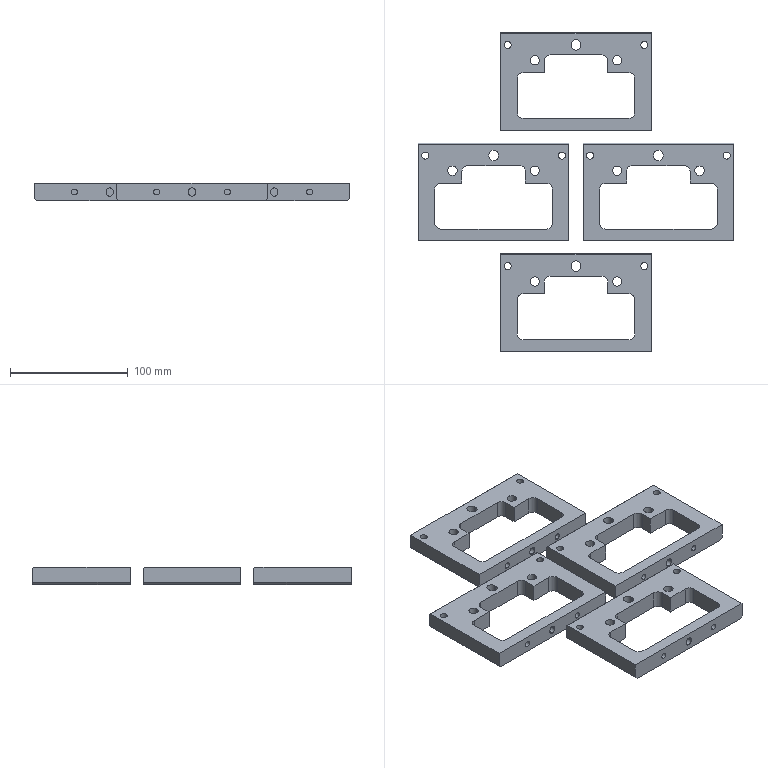NC program | NX | posted with a generic post | part box 268 x 271 x 15 mm
Lines 1946 to 2286 of 2286:
(PLANAR_MILL_1_COPY , TOOL : D6A45)
N3878 T07 M6
N3880 G54
N3882 G17 G0 G90 X31.063 Y-0.325 B0. C0. S9500 M3
N3884 G43 Z30. H7
N3886 Z0.
N3888 G94 G1 X31.1 Y-0.259 Z-0.02 F1250.
N3890 Y0. Z-0.09
N3892 Y0.259 Z-0.159
N3894 X30.799 Y0.799 Z-0.325
N3896 X30.259 Y1.1 Z-0.491
N3898 X29.741 Z-0.629
N3900 X29.201 Y0.799 Z-0.795
N3902 X28.9 Y0.259 Z-0.961
N3904 Y-0.259 Z-1.099
N3906 X29.201 Y-0.799 Z-1.265
N3908 X29.741 Y-1.1 Z-1.431
N3910 X30. Z-1.5
N3912 G3 X31.1 Y0. R1.1
N3914 X30. Y-1.1 R-1.1
N3916 X30.866 Y-0.6 R1.
N3918 G1 Z0.
N3920 G0 Z30.
N3922 X0.38 Y-0.626
N3924 Z0.
N3926 G1 Z-1.5
N3928 X1.1 Y-0.866
N3930 G3 X1.6 Y0. R1.
N3932 G1 Y0.5
N3934 G3 X0. Y2.1 R1.6
N3936 X-1.6 Y0.5 R1.6
N3938 G1 Y-0.5
N3940 G3 X0. Y-2.1 R1.6
N3942 X1.6 Y-0.5 R1.6
N3944 G1 Y0.
N3946 G3 X1.1 Y0.866 R1.
N3948 G1 X0.38 Y0.626
N3950 Z0.
N3952 G0 Z30.
N3954 X-28.937 Y-0.325
N3956 Z0.
N3958 G1 X-28.9 Y-0.259 Z-0.02
N3960 Y0. Z-0.09
N3962 Y0.259 Z-0.159
N3964 X-29.201 Y0.799 Z-0.325
N3966 X-29.741 Y1.1 Z-0.491
N3968 X-30.259 Z-0.629
N3970 X-30.799 Y0.799 Z-0.795
N3972 X-31.1 Y0.259 Z-0.961
N3974 Y-0.259 Z-1.099
N3976 X-30.799 Y-0.799 Z-1.265
N3978 X-30.259 Y-1.1 Z-1.431
N3980 X-30. Z-1.5
N3982 G3 X-28.9 Y0. R1.1
N3984 X-30. Y-1.1 R-1.1
N3986 X-29.134 Y-0.6 R1.
N3988 G1 Z0.
N3990 G0 Z30.
N3992 M5
(TOOLCOMP4_COPY , TOOL : D4)
N3994 T04 M6
N3996 G54
N3998 G17 G0 G90 X-0.499 Y0.731 B0. C0. S9500 M3
N4000 G43 Z30. H4
N4002 Z-0.333
N4004 G94 G1 Z-1.333 F1000.
N4006 G41 X-0.75 Y0.846 D4
N4008 G3 X-0.95 Y0.5 R0.4
N4010 G1 Y-0.5 F1200.
N4012 G3 X0. Y-1.45 R0.95
N4014 X0.95 Y-0.5 R0.95
N4016 G1 Y0.5
N4018 G3 X0. Y1.45 R0.95
N4020 X-0.95 Y0.5 R0.95
N4022 G1 Y-0.354 Z-1.524
N4024 X-0.944 Y-0.496 Z-1.556
N4026 X-0.933 Y-0.637 Z-1.587
N4028 X-0.91 Y-0.741 Z-1.611
N4030 X-0.897 Y-0.793 Z-1.623
N4032 X-0.882 Y-0.831 Z-1.632
N4034 X-0.85 Y-0.906 Z-1.651
N4036 X-0.795 Y-1.004 Z-1.676
N4038 X-0.765 Y-1.052 Z-1.689
N4040 X-0.741 Y-1.081 Z-1.697
N4042 X-0.692 Y-1.138 Z-1.714
N4044 X-0.609 Y-1.217 Z-1.74
N4046 X-0.566 Y-1.254 Z-1.753
N4048 X-0.536 Y-1.276 Z-1.761
N4050 X-0.473 Y-1.314 Z-1.778
N4052 X-0.365 Y-1.367 Z-1.805
N4054 X-0.31 Y-1.39 Z-1.818
N4056 X-0.278 Y-1.401 Z-1.826
N4058 X-0.212 Y-1.417 Z-1.841
N4060 X-0.09 Y-1.436 Z-1.869
N4062 X0.003 Y-1.443 Z-1.89
N4064 X0.069 Y-1.439 Z-1.905
N4066 X0.193 Y-1.421 Z-1.933
N4068 X0.284 Y-1.399 Z-1.954
N4070 X0.342 Y-1.377 Z-1.968
N4072 X0.457 Y-1.323 Z-1.997
N4074 X0.537 Y-1.274 Z-2.018
N4076 X0.586 Y-1.237 Z-2.032
N4078 X0.677 Y-1.157 Z-2.059
N4080 X0.738 Y-1.086 Z-2.08
N4082 X0.778 Y-1.031 Z-2.095
N4084 X0.838 Y-0.933 Z-2.121
N4086 X0.875 Y-0.847 Z-2.142
N4088 X0.901 Y-0.778 Z-2.159
N4090 X0.926 Y-0.672 Z-2.183
N4092 X0.935 Y-0.615 Z-2.196
N4094 X0.944 Y-0.5 Z-2.222
N4096 X0.95 Y-0.358 Z-2.254
N4098 Y0.354 Z-2.413
N4100 X0.944 Y0.496 Z-2.444
N4102 X0.933 Y0.637 Z-2.476
N4104 X0.91 Y0.741 Z-2.5
N4106 X0.897 Y0.793 Z-2.512
N4108 X0.85 Y0.906 Z-2.54
N4110 X0.798 Y1. Z-2.564
N4112 X0.77 Y1.045 Z-2.576
N4114 X0.744 Y1.077 Z-2.585
N4116 X0.692 Y1.138 Z-2.603
N4118 X0.588 Y1.235 Z-2.635
N4120 X0.477 Y1.321 Z-2.667
N4122 G3 X-0.95 Y0.5 R0.95
N4124 G1 Y-0.354 Z-2.857
N4126 X-0.944 Y-0.496 Z-2.889
N4128 X-0.933 Y-0.637 Z-2.921
N4130 X-0.909 Y-0.742 Z-2.945
N4132 X-0.897 Y-0.795 Z-2.957
N4134 X-0.85 Y-0.906 Z-2.984
N4136 X-0.795 Y-1.004 Z-3.009
N4138 X-0.766 Y-1.052 Z-3.022
N4140 X-0.692 Y-1.138 Z-3.048
N4142 X-0.609 Y-1.217 Z-3.073
N4144 X-0.566 Y-1.254 Z-3.086
N4146 X-0.536 Y-1.275 Z-3.094
N4148 X-0.473 Y-1.314 Z-3.111
N4150 X-0.365 Y-1.367 Z-3.138
N4152 X-0.31 Y-1.39 Z-3.151
N4154 X-0.278 Y-1.401 Z-3.159
N4156 X-0.212 Y-1.417 Z-3.175
N4158 X-0.091 Y-1.436 Z-3.202
N4160 X0.003 Y-1.443 Z-3.223
N4162 X0.068 Y-1.438 Z-3.238
N4164 X0.192 Y-1.421 Z-3.266
N4166 X0.284 Y-1.399 Z-3.287
N4168 X0.342 Y-1.376 Z-3.302
N4170 X0.457 Y-1.323 Z-3.33
N4172 X0.537 Y-1.275 Z-3.351
N4174 X0.586 Y-1.237 Z-3.365
N4176 X0.676 Y-1.157 Z-3.392
N4178 X0.737 Y-1.086 Z-3.413
N4180 X0.778 Y-1.031 Z-3.429
N4182 X0.838 Y-0.933 Z-3.454
N4184 X0.874 Y-0.847 Z-3.475
N4186 X0.901 Y-0.778 Z-3.492
N4188 X0.926 Y-0.673 Z-3.517
N4190 X0.935 Y-0.616 Z-3.53
N4192 X0.944 Y-0.5 Z-3.556
N4194 X0.95 Y-0.358 Z-3.587
N4196 Y0.354 Z-3.746
N4198 X0.944 Y0.496 Z-3.778
N4200 X0.933 Y0.637 Z-3.81
N4202 X0.909 Y0.742 Z-3.834
N4204 X0.897 Y0.795 Z-3.846
N4206 X0.85 Y0.906 Z-3.873
N4208 X0.798 Y0.999 Z-3.897
N4210 X0.77 Y1.045 Z-3.909
N4212 X0.745 Y1.077 Z-3.918
N4214 X0.692 Y1.138 Z-3.937
N4216 X0.588 Y1.234 Z-3.968
N4218 X0.477 Y1.321 Z-4.
N4220 G3 X-0.95 Y0.5 R0.95
N4222 G1 Y-0.354 Z-4.19
N4224 X-0.944 Y-0.496 Z-4.222
N4226 X-0.933 Y-0.637 Z-4.254
N4228 X-0.909 Y-0.742 Z-4.278
N4230 X-0.897 Y-0.794 Z-4.29
N4232 X-0.85 Y-0.906 Z-4.317
N4234 X-0.795 Y-1.004 Z-4.343
N4236 X-0.766 Y-1.051 Z-4.355
N4238 X-0.692 Y-1.138 Z-4.381
N4240 X-0.609 Y-1.217 Z-4.407
N4242 X-0.566 Y-1.254 Z-4.419
N4244 X-0.536 Y-1.275 Z-4.428
N4246 X-0.473 Y-1.314 Z-4.444
N4248 X-0.366 Y-1.367 Z-4.471
N4250 X-0.311 Y-1.389 Z-4.485
N4252 X-0.278 Y-1.4 Z-4.492
N4254 X-0.211 Y-1.417 Z-4.508
N4256 X-0.091 Y-1.436 Z-4.535
N4258 X0.002 Y-1.444 Z-4.556
N4260 X0.068 Y-1.438 Z-4.571
N4262 X0.195 Y-1.421 Z-4.6
N4264 X0.286 Y-1.399 Z-4.621
N4266 X0.342 Y-1.376 Z-4.635
N4268 X0.459 Y-1.322 Z-4.664
N4270 X0.539 Y-1.273 Z-4.685
N4272 X0.586 Y-1.237 Z-4.698
N4274 X0.677 Y-1.155 Z-4.726
N4276 X0.738 Y-1.084 Z-4.747
N4278 X0.778 Y-1.031 Z-4.762
N4280 X0.838 Y-0.934 Z-4.787
N4282 X0.874 Y-0.847 Z-4.809
N4284 X0.901 Y-0.778 Z-4.825
N4286 X0.926 Y-0.674 Z-4.85
N4288 X0.934 Y-0.616 Z-4.863
N4290 X0.944 Y-0.5 Z-4.889
N4292 X0.95 Y-0.358 Z-4.921
N4294 Y0.354 Z-5.079
N4296 X0.944 Y0.496 Z-5.111
N4298 X0.933 Y0.637 Z-5.143
N4300 X0.91 Y0.742 Z-5.167
N4302 X0.896 Y0.794 Z-5.179
N4304 X0.85 Y0.906 Z-5.206
N4306 X0.798 Y0.999 Z-5.23
N4308 X0.77 Y1.044 Z-5.242
N4310 X0.745 Y1.076 Z-5.252
N4312 X0.692 Y1.138 Z-5.27
N4314 X0.589 Y1.235 Z-5.302
N4316 X0.477 Y1.321 Z-5.333
N4318 G3 X-0.95 Y0.5 R0.95
N4320 G1 Y-0.354 Z-5.524
N4322 X-0.944 Y-0.496 Z-5.556
N4324 X-0.933 Y-0.637 Z-5.587
N4326 X-0.909 Y-0.742 Z-5.611
N4328 X-0.896 Y-0.794 Z-5.624
N4330 X-0.85 Y-0.906 Z-5.651
N4332 X-0.795 Y-1.003 Z-5.676
N4334 X-0.766 Y-1.051 Z-5.689
N4336 X-0.742 Y-1.08 Z-5.697
N4338 X-0.692 Y-1.138 Z-5.714
N4340 X-0.608 Y-1.218 Z-5.74
N4342 X-0.564 Y-1.255 Z-5.753
N4344 X-0.534 Y-1.276 Z-5.761
N4346 X-0.473 Y-1.313 Z-5.778
N4348 X-0.366 Y-1.366 Z-5.804
N4350 X-0.311 Y-1.389 Z-5.818
N4352 X-0.279 Y-1.4 Z-5.826
N4354 X-0.211 Y-1.417 Z-5.841
N4356 X-0.092 Y-1.436 Z-5.868
N4358 X0.002 Y-1.443 Z-5.89
N4360 X0.068 Y-1.438 Z-5.905
N4362 X0.194 Y-1.421 Z-5.933
N4364 X0.285 Y-1.399 Z-5.954
N4366 X0.342 Y-1.376 Z-5.968
N4368 X0.458 Y-1.322 Z-5.997
N4370 X0.538 Y-1.274 Z-6.018
N4372 X0.586 Y-1.237 Z-6.032
N4374 X0.677 Y-1.155 Z-6.059
N4376 X0.738 Y-1.084 Z-6.08
N4378 X0.778 Y-1.031 Z-6.095
N4380 X0.837 Y-0.934 Z-6.121
N4382 X0.874 Y-0.848 Z-6.142
N4384 X0.9 Y-0.778 Z-6.159
N4386 X0.918 Y-0.707 Z-6.175
N4388 X0.926 Y-0.671 Z-6.184
N4390 X0.935 Y-0.615 Z-6.196
N4392 X0.943 Y-0.5 Z-6.222
N4394 X0.95 Y-0.358 Z-6.254
N4396 Y0.354 Z-6.413
N4398 X0.944 Y0.496 Z-6.444
N4400 X0.933 Y0.637 Z-6.476
N4402 X0.909 Y0.742 Z-6.5
N4404 X0.896 Y0.794 Z-6.512
N4406 X0.85 Y0.906 Z-6.54
N4408 X0.798 Y0.998 Z-6.564
N4410 X0.77 Y1.044 Z-6.576
N4412 X0.745 Y1.076 Z-6.585
N4414 X0.692 Y1.138 Z-6.603
N4416 X0.588 Y1.235 Z-6.635
N4418 X0.477 Y1.321 Z-6.667
N4420 G3 X-0.95 Y0.5 R0.95
N4422 G1 Y-0.354 Z-6.857
N4424 X-0.944 Y-0.496 Z-6.889
N4426 X-0.933 Y-0.637 Z-6.921
N4428 X-0.909 Y-0.742 Z-6.945
N4430 X-0.896 Y-0.794 Z-6.957
N4432 X-0.85 Y-0.906 Z-6.984
N4434 X-0.795 Y-1.003 Z-7.009
N4436 X-0.766 Y-1.051 Z-7.022
N4438 X-0.742 Y-1.08 Z-7.03
N4440 X-0.692 Y-1.138 Z-7.048
N4442 X-0.608 Y-1.217 Z-7.073
N4444 X-0.565 Y-1.255 Z-7.086
N4446 X-0.535 Y-1.275 Z-7.095
N4448 X-0.473 Y-1.313 Z-7.111
N4450 X-0.366 Y-1.366 Z-7.138
N4452 X-0.312 Y-1.389 Z-7.151
N4454 X-0.279 Y-1.4 Z-7.159
N4456 X-0.211 Y-1.417 Z-7.175
N4458 X-0.089 Y-1.436 Z-7.202
N4460 X0.004 Y-1.443 Z-7.223
N4462 X0.068 Y-1.438 Z-7.238
N4464 X0.194 Y-1.421 Z-7.266
N4466 X0.285 Y-1.399 Z-7.288
N4468 X0.342 Y-1.376 Z-7.302
N4470 X0.458 Y-1.322 Z-7.33
N4472 X0.537 Y-1.274 Z-7.351
N4474 X0.586 Y-1.236 Z-7.365
N4476 X0.676 Y-1.155 Z-7.392
N4478 X0.737 Y-1.084 Z-7.413
N4480 X0.778 Y-1.031 Z-7.429
N4482 X0.837 Y-0.934 Z-7.454
N4484 X0.874 Y-0.848 Z-7.475
N4486 X0.9 Y-0.778 Z-7.492
N4488 X0.917 Y-0.707 Z-7.508
N4490 X0.926 Y-0.672 Z-7.517
N4492 X0.934 Y-0.615 Z-7.53
N4494 X0.943 Y-0.5 Z-7.556
N4496 X0.95 Y-0.358 Z-7.587
N4498 Y0.354 Z-7.746
N4500 X0.944 Y0.496 Z-7.778
N4502 X0.933 Y0.637 Z-7.81
N4504 X0.909 Y0.742 Z-7.834
N4506 X0.896 Y0.794 Z-7.846
N4508 X0.85 Y0.906 Z-7.873
N4510 X0.798 Y0.998 Z-7.897
N4512 X0.77 Y1.043 Z-7.909
N4514 X0.745 Y1.076 Z-7.918
N4516 X0.692 Y1.138 Z-7.937
N4518 X0.588 Y1.234 Z-7.968
N4520 X0.477 Y1.321 Z-8.
N4522 G3 X-0.95 Y0.5 R0.95
N4524 G1 Y-0.5
N4526 G3 X0. Y-1.45 R0.95
N4528 X0.95 Y-0.5 R0.95
N4530 G1 Y0.5
N4532 G3 X0.477 Y1.321 R0.95
N4534 X0.077 Y1.323 R0.4
N4536 G40
N4538 G1 X0.051 Y1.048
N4540 Z-7.
N4542 G0 Z30.
N4544 M5
N4546 M2